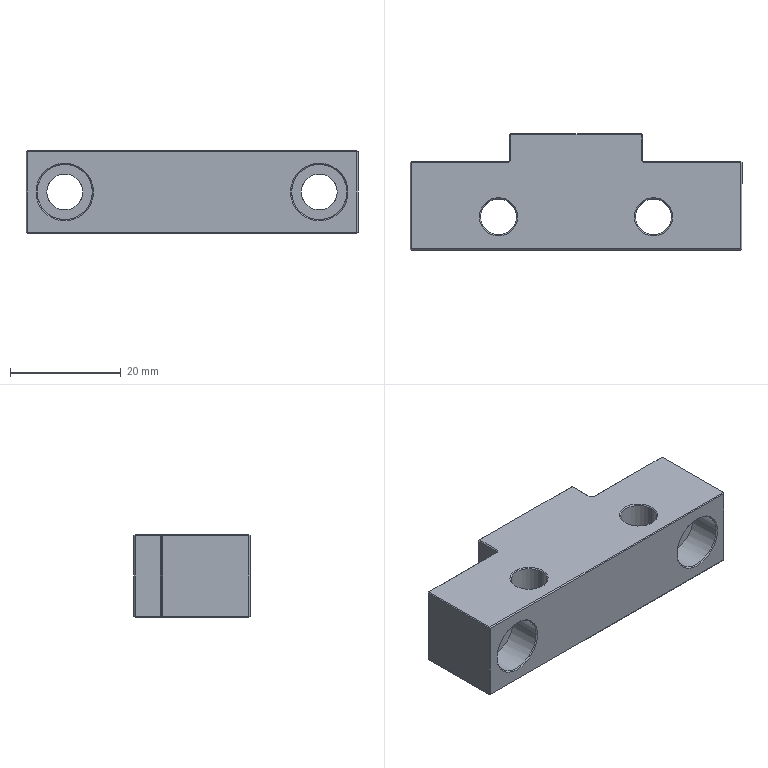Part | 1 solid | 80 faces | box 60 x 21 x 15 mm | volume 13587 mm3 | plane 52 | cone 16 | cylinder 12 | commonest cylinder face diameters 6.5 x8 10 x4